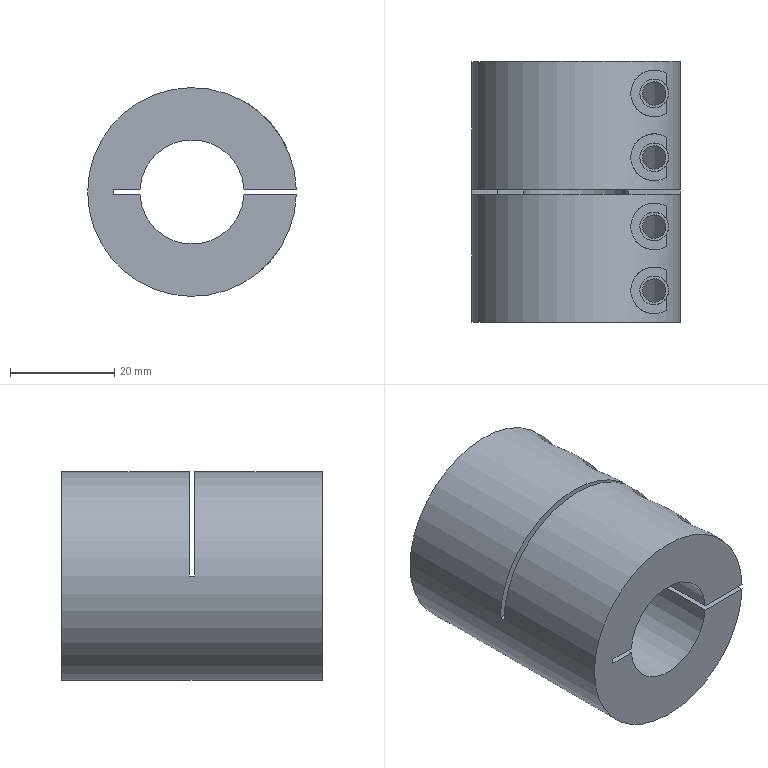Part | NX | features SIMPLE HOLE 14, DATUM_CSYS 6, SYMBOLIC_THREAD 6, SKETCH 5, EXTRUDE 4, HOLE PACKAGE 3, ASSOCIATIVE_INTERSECTION 1, SWP104 1 | 1 solid | 40 faces | box 39.994 x 50 x 40 mm | volume 43416 mm3 | cylinder 20 | plane 16 | spline 4 | commonest cylinder face diameters 40 x5 4.5 x4 5.5 x4 9 x4 20 x3